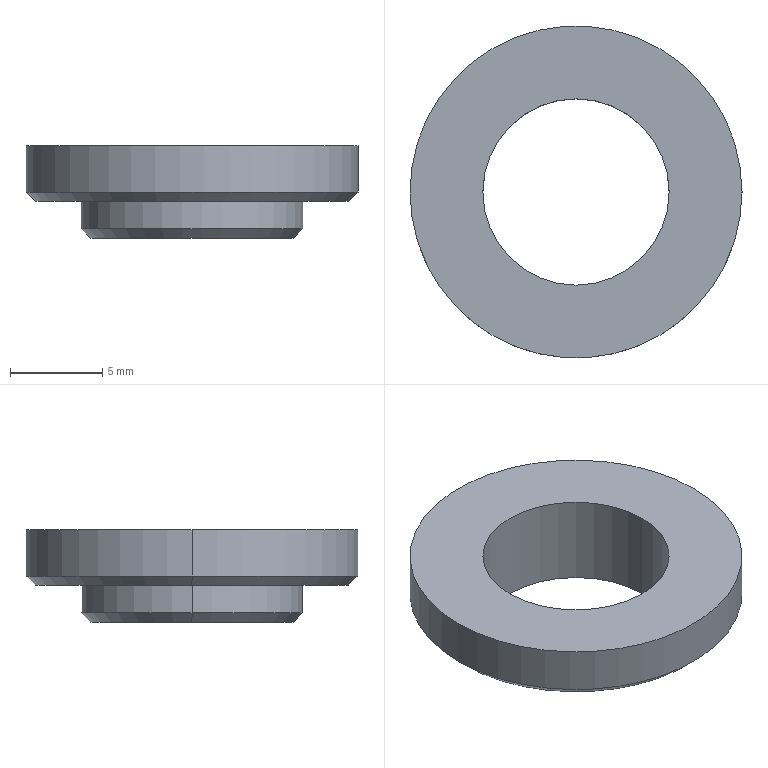Part | SolidWorks | features BaseBody 1 | 1 solid | 13 faces | box 18 x 18 x 5 mm | volume 577.49 mm3 | cylinder 6 | cone 4 | plane 3 | commonest cylinder face diameters 10.1 x2 12 x2 18 x2
STEP:
#1=CARTESIAN_POINT('',(-8.5,0.,2.));
#2=VERTEX_POINT('',#1);
#3=CARTESIAN_POINT('',(8.5,0.,2.));
#4=VERTEX_POINT('',#3);
#5=CARTESIAN_POINT('',(0.,0.,2.));
#6=DIRECTION('',(0.,0.,-1.));
#7=DIRECTION('',(-1.,0.,0.));
#8=AXIS2_PLACEMENT_3D('',#5,#6,#7);
#9=CIRCLE('',#8,8.5);
#10=EDGE_CURVE('',#2,#4,#9,.T.);
#11=ORIENTED_EDGE('',*,*,#10,.F.);
#12=CARTESIAN_POINT('',(-9.,0.,2.5));
#13=VERTEX_POINT('',#12);
#14=CARTESIAN_POINT('',(-8.5,0.,2.));
#15=DIRECTION('',(-0.7071,0.,0.7071));
#16=VECTOR('',#15,1000.);
#17=LINE('',#14,#16);
#18=EDGE_CURVE('',#2,#13,#17,.T.);
#19=ORIENTED_EDGE('',*,*,#18,.T.);
#20=CARTESIAN_POINT('',(9.,0.,2.5));
#21=VERTEX_POINT('',#20);
#22=CARTESIAN_POINT('',(0.,0.,2.5));
#23=DIRECTION('',(0.,0.,1.));
#24=DIRECTION('',(-1.,0.,0.));
#25=AXIS2_PLACEMENT_3D('',#22,#23,#24);
#26=CIRCLE('',#25,9.);
#27=EDGE_CURVE('',#21,#13,#26,.T.);
#28=ORIENTED_EDGE('',*,*,#27,.F.);
#29=CARTESIAN_POINT('',(8.5,0.,2.));
#30=DIRECTION('',(0.7071,0.,0.7071));
#31=VECTOR('',#30,1000.);
#32=LINE('',#29,#31);
#33=EDGE_CURVE('',#4,#21,#32,.T.);
#34=ORIENTED_EDGE('',*,*,#33,.F.);
#35=EDGE_LOOP('',(#11,#19,#28,#34));
#36=FACE_OUTER_BOUND('',#35,.T.);
#37=CARTESIAN_POINT('',(0.,0.,2.));
#38=DIRECTION('',(0.,0.,1.));
#39=DIRECTION('',(1.,0.,0.));
#40=AXIS2_PLACEMENT_3D('',#37,#38,#39);
#41=CONICAL_SURFACE('',#40,8.5,0.7854);
#42=ADVANCED_FACE('',(#36),#41,.T.);
#43=CARTESIAN_POINT('',(-5.5,0.,0.));
#44=VERTEX_POINT('',#43);
#45=CARTESIAN_POINT('',(5.5,0.,0.));
#46=VERTEX_POINT('',#45);
#47=CARTESIAN_POINT('',(0.,0.,0.));
#48=DIRECTION('',(0.,0.,-1.));
#49=DIRECTION('',(1.,0.,0.));
#50=AXIS2_PLACEMENT_3D('',#47,#48,#49);
#51=CIRCLE('',#50,5.5);
#52=EDGE_CURVE('',#44,#46,#51,.T.);
#53=ORIENTED_EDGE('',*,*,#52,.F.);
#54=CARTESIAN_POINT('',(-6.,0.,0.5));
#55=VERTEX_POINT('',#54);
#56=CARTESIAN_POINT('',(-5.5,0.,0.));
#57=DIRECTION('',(-0.7071,0.,0.7071));
#58=VECTOR('',#57,1000.);
#59=LINE('',#56,#58);
#60=EDGE_CURVE('',#44,#55,#59,.T.);
#61=ORIENTED_EDGE('',*,*,#60,.T.);
#62=CARTESIAN_POINT('',(6.,0.,0.5));
#63=VERTEX_POINT('',#62);
#64=CARTESIAN_POINT('',(0.,0.,0.5));
#65=DIRECTION('',(0.,0.,1.));
#66=DIRECTION('',(1.,0.,0.));
#67=AXIS2_PLACEMENT_3D('',#64,#65,#66);
#68=CIRCLE('',#67,6.);
#69=EDGE_CURVE('',#63,#55,#68,.T.);
#70=ORIENTED_EDGE('',*,*,#69,.F.);
#71=CARTESIAN_POINT('',(5.5,0.,0.));
#72=DIRECTION('',(0.7071,0.,0.7071));
#73=VECTOR('',#72,1000.);
#74=LINE('',#71,#73);
#75=EDGE_CURVE('',#46,#63,#74,.T.);
#76=ORIENTED_EDGE('',*,*,#75,.F.);
#77=EDGE_LOOP('',(#53,#61,#70,#76));
#78=FACE_OUTER_BOUND('',#77,.T.);
#79=CARTESIAN_POINT('',(0.,0.,0.));
#80=DIRECTION('',(0.,0.,1.));
#81=DIRECTION('',(1.,0.,0.));
#82=AXIS2_PLACEMENT_3D('',#79,#80,#81);
#83=CONICAL_SURFACE('',#82,5.5,0.7854);
#84=ADVANCED_FACE('',(#78),#83,.T.);
#85=CARTESIAN_POINT('',(-6.,0.,2.));
#86=VERTEX_POINT('',#85);
#87=CARTESIAN_POINT('',(6.,0.,2.));
#88=VERTEX_POINT('',#87);
#89=CARTESIAN_POINT('',(0.,0.,2.));
#90=DIRECTION('',(0.,0.,-1.));
#91=DIRECTION('',(-1.,0.,0.));
#92=AXIS2_PLACEMENT_3D('',#89,#90,#91);
#93=CIRCLE('',#92,6.);
#94=EDGE_CURVE('',#86,#88,#93,.T.);
#95=ORIENTED_EDGE('',*,*,#94,.T.);
#96=CARTESIAN_POINT('',(6.,0.,2.));
#97=DIRECTION('',(0.,0.,-1.));
#98=VECTOR('',#97,1000.);
#99=LINE('',#96,#98);
#100=EDGE_CURVE('',#88,#63,#99,.T.);
#101=ORIENTED_EDGE('',*,*,#100,.T.);
#102=ORIENTED_EDGE('',*,*,#69,.T.);
#103=CARTESIAN_POINT('',(-6.,0.,2.));
#104=DIRECTION('',(0.,0.,-1.));
#105=VECTOR('',#104,1000.);
#106=LINE('',#103,#105);
#107=EDGE_CURVE('',#86,#55,#106,.T.);
#108=ORIENTED_EDGE('',*,*,#107,.F.);
#109=EDGE_LOOP('',(#95,#101,#102,#108));
#110=FACE_OUTER_BOUND('',#109,.T.);
#111=CARTESIAN_POINT('',(0.,0.,2.));
#112=DIRECTION('',(0.,0.,-1.));
#113=DIRECTION('',(-1.,0.,0.));
#114=AXIS2_PLACEMENT_3D('',#111,#112,#113);
#115=CYLINDRICAL_SURFACE('',#114,6.);
#116=ADVANCED_FACE('',(#110),#115,.T.);
#117=CARTESIAN_POINT('',(-5.05,0.,5.));
#118=VERTEX_POINT('',#117);
#119=CARTESIAN_POINT('',(5.05,0.,5.));
#120=VERTEX_POINT('',#119);
#121=CARTESIAN_POINT('',(0.,0.,5.));
#122=DIRECTION('',(0.,0.,1.));
#123=DIRECTION('',(1.,0.,0.));
#124=AXIS2_PLACEMENT_3D('',#121,#122,#123);
#125=CIRCLE('',#124,5.05);
#126=EDGE_CURVE('',#118,#120,#125,.T.);
#127=ORIENTED_EDGE('',*,*,#126,.T.);
#128=CARTESIAN_POINT('',(5.05,0.,0.));
#129=VERTEX_POINT('',#128);
#130=CARTESIAN_POINT('',(5.05,0.,5.));
#131=DIRECTION('',(0.,0.,-1.));
#132=VECTOR('',#131,1000.);
#133=LINE('',#130,#132);
#134=EDGE_CURVE('',#120,#129,#133,.T.);
#135=ORIENTED_EDGE('',*,*,#134,.T.);
#136=CARTESIAN_POINT('',(-5.05,0.,0.));
#137=VERTEX_POINT('',#136);
#138=CARTESIAN_POINT('',(0.,0.,0.));
#139=DIRECTION('',(0.,0.,1.));
#140=DIRECTION('',(1.,0.,0.));
#141=AXIS2_PLACEMENT_3D('',#138,#139,#140);
#142=CIRCLE('',#141,5.05);
#143=EDGE_CURVE('',#137,#129,#142,.T.);
#144=ORIENTED_EDGE('',*,*,#143,.F.);
#145=CARTESIAN_POINT('',(-5.05,0.,5.));
#146=DIRECTION('',(0.,0.,-1.));
#147=VECTOR('',#146,1000.);
#148=LINE('',#145,#147);
#149=EDGE_CURVE('',#118,#137,#148,.T.);
#150=ORIENTED_EDGE('',*,*,#149,.F.);
#151=EDGE_LOOP('',(#127,#135,#144,#150));
#152=FACE_OUTER_BOUND('',#151,.T.);
#153=CARTESIAN_POINT('',(0.,0.,5.));
#154=DIRECTION('',(0.,0.,-1.));
#155=DIRECTION('',(-1.,0.,0.));
#156=AXIS2_PLACEMENT_3D('',#153,#154,#155);
#157=CYLINDRICAL_SURFACE('',#156,5.05);
#158=ADVANCED_FACE('',(#152),#157,.F.);
#159=CARTESIAN_POINT('',(9.,0.,5.));
#160=VERTEX_POINT('',#159);
#161=CARTESIAN_POINT('',(-9.,0.,5.));
#162=VERTEX_POINT('',#161);
#163=CARTESIAN_POINT('',(0.,0.,5.));
#164=DIRECTION('',(0.,0.,1.));
#165=DIRECTION('',(1.,0.,0.));
#166=AXIS2_PLACEMENT_3D('',#163,#164,#165);
#167=CIRCLE('',#166,9.);
#168=EDGE_CURVE('',#160,#162,#167,.T.);
#169=ORIENTED_EDGE('',*,*,#168,.F.);
#170=CARTESIAN_POINT('',(9.,0.,5.));
#171=DIRECTION('',(0.,0.,-1.));
#172=VECTOR('',#171,1000.);
#173=LINE('',#170,#172);
#174=EDGE_CURVE('',#160,#21,#173,.T.);
#175=ORIENTED_EDGE('',*,*,#174,.T.);
#176=ORIENTED_EDGE('',*,*,#27,.T.);
#177=CARTESIAN_POINT('',(-9.,0.,5.));
#178=DIRECTION('',(0.,0.,-1.));
#179=VECTOR('',#178,1000.);
#180=LINE('',#177,#179);
#181=EDGE_CURVE('',#162,#13,#180,.T.);
#182=ORIENTED_EDGE('',*,*,#181,.F.);
#183=EDGE_LOOP('',(#169,#175,#176,#182));
#184=FACE_OUTER_BOUND('',#183,.T.);
#185=CARTESIAN_POINT('',(0.,0.,5.));
#186=DIRECTION('',(0.,0.,-1.));
#187=DIRECTION('',(-1.,0.,0.));
#188=AXIS2_PLACEMENT_3D('',#185,#186,#187);
#189=CYLINDRICAL_SURFACE('',#188,9.);
#190=ADVANCED_FACE('',(#184),#189,.T.);
#191=ORIENTED_EDGE('',*,*,#94,.F.);
#192=CARTESIAN_POINT('',(0.,0.,2.));
#193=DIRECTION('',(0.,0.,-1.));
#194=DIRECTION('',(-1.,0.,0.));
#195=AXIS2_PLACEMENT_3D('',#192,#193,#194);
#196=CIRCLE('',#195,6.);
#197=EDGE_CURVE('',#88,#86,#196,.T.);
#198=ORIENTED_EDGE('',*,*,#197,.F.);
#199=EDGE_LOOP('',(#191,#198));
#200=FACE_BOUND('',#199,.T.);
#201=CARTESIAN_POINT('',(0.,0.,2.));
#202=DIRECTION('',(0.,0.,-1.));
#203=DIRECTION('',(-1.,0.,0.));
#204=AXIS2_PLACEMENT_3D('',#201,#202,#203);
#205=CIRCLE('',#204,8.5);
#206=EDGE_CURVE('',#4,#2,#205,.T.);
#207=ORIENTED_EDGE('',*,*,#206,.T.);
#208=ORIENTED_EDGE('',*,*,#10,.T.);
#209=EDGE_LOOP('',(#207,#208));
#210=FACE_OUTER_BOUND('',#209,.T.);
#211=CARTESIAN_POINT('',(0.,0.,2.));
#212=DIRECTION('',(0.,0.,-1.));
#213=DIRECTION('',(0.,-1.,0.));
#214=AXIS2_PLACEMENT_3D('',#211,#212,#213);
#215=PLANE('',#214);
#216=ADVANCED_FACE('',(#200,#210),#215,.T.);
#217=ORIENTED_EDGE('',*,*,#126,.F.);
#218=CARTESIAN_POINT('',(0.,0.,5.));
#219=DIRECTION('',(0.,0.,1.));
#220=DIRECTION('',(1.,0.,0.));
#221=AXIS2_PLACEMENT_3D('',#218,#219,#220);
#222=CIRCLE('',#221,5.05);
#223=EDGE_CURVE('',#120,#118,#222,.T.);
#224=ORIENTED_EDGE('',*,*,#223,.F.);
#225=EDGE_LOOP('',(#217,#224));
#226=FACE_BOUND('',#225,.T.);
#227=CARTESIAN_POINT('',(0.,0.,5.));
#228=DIRECTION('',(0.,0.,1.));
#229=DIRECTION('',(1.,0.,0.));
#230=AXIS2_PLACEMENT_3D('',#227,#228,#229);
#231=CIRCLE('',#230,9.);
#232=EDGE_CURVE('',#162,#160,#231,.T.);
#233=ORIENTED_EDGE('',*,*,#232,.T.);
#234=ORIENTED_EDGE('',*,*,#168,.T.);
#235=EDGE_LOOP('',(#233,#234));
#236=FACE_OUTER_BOUND('',#235,.T.);
#237=CARTESIAN_POINT('',(0.,0.,5.));
#238=DIRECTION('',(0.,0.,1.));
#239=DIRECTION('',(1.,0.,0.));
#240=AXIS2_PLACEMENT_3D('',#237,#238,#239);
#241=PLANE('',#240);
#242=ADVANCED_FACE('',(#226,#236),#241,.T.);
#243=ORIENTED_EDGE('',*,*,#143,.T.);
#244=CARTESIAN_POINT('',(0.,0.,0.));
#245=DIRECTION('',(0.,0.,1.));
#246=DIRECTION('',(1.,0.,0.));
#247=AXIS2_PLACEMENT_3D('',#244,#245,#246);
#248=CIRCLE('',#247,5.05);
#249=EDGE_CURVE('',#129,#137,#248,.T.);
#250=ORIENTED_EDGE('',*,*,#249,.T.);
#251=EDGE_LOOP('',(#243,#250));
#252=FACE_BOUND('',#251,.T.);
#253=CARTESIAN_POINT('',(0.,0.,0.));
#254=DIRECTION('',(0.,0.,-1.));
#255=DIRECTION('',(1.,0.,0.));
#256=AXIS2_PLACEMENT_3D('',#253,#254,#255);
#257=CIRCLE('',#256,5.5);
#258=EDGE_CURVE('',#46,#44,#257,.T.);
#259=ORIENTED_EDGE('',*,*,#258,.T.);
#260=ORIENTED_EDGE('',*,*,#52,.T.);
#261=EDGE_LOOP('',(#259,#260));
#262=FACE_OUTER_BOUND('',#261,.T.);
#263=CARTESIAN_POINT('',(0.,0.,0.));
#264=DIRECTION('',(0.,0.,1.));
#265=DIRECTION('',(1.,0.,0.));
#266=AXIS2_PLACEMENT_3D('',#263,#264,#265);
#267=PLANE('',#266);
#268=ADVANCED_FACE('',(#252,#262),#267,.F.);
#269=ORIENTED_EDGE('',*,*,#174,.F.);
#270=ORIENTED_EDGE('',*,*,#232,.F.);
#271=ORIENTED_EDGE('',*,*,#181,.T.);
#272=CARTESIAN_POINT('',(0.,0.,2.5));
#273=DIRECTION('',(0.,0.,1.));
#274=DIRECTION('',(-1.,0.,0.));
#275=AXIS2_PLACEMENT_3D('',#272,#273,#274);
#276=CIRCLE('',#275,9.);
#277=EDGE_CURVE('',#13,#21,#276,.T.);
#278=ORIENTED_EDGE('',*,*,#277,.T.);
#279=EDGE_LOOP('',(#269,#270,#271,#278));
#280=FACE_OUTER_BOUND('',#279,.T.);
#281=CARTESIAN_POINT('',(0.,0.,5.));
#282=DIRECTION('',(0.,0.,-1.));
#283=DIRECTION('',(-1.,0.,0.));
#284=AXIS2_PLACEMENT_3D('',#281,#282,#283);
#285=CYLINDRICAL_SURFACE('',#284,9.);
#286=ADVANCED_FACE('',(#280),#285,.T.);
#287=ORIENTED_EDGE('',*,*,#134,.F.);
#288=ORIENTED_EDGE('',*,*,#223,.T.);
#289=ORIENTED_EDGE('',*,*,#149,.T.);
#290=ORIENTED_EDGE('',*,*,#249,.F.);
#291=EDGE_LOOP('',(#287,#288,#289,#290));
#292=FACE_OUTER_BOUND('',#291,.T.);
#293=CARTESIAN_POINT('',(0.,0.,5.));
#294=DIRECTION('',(0.,0.,-1.));
#295=DIRECTION('',(-1.,0.,0.));
#296=AXIS2_PLACEMENT_3D('',#293,#294,#295);
#297=CYLINDRICAL_SURFACE('',#296,5.05);
#298=ADVANCED_FACE('',(#292),#297,.F.);
#299=ORIENTED_EDGE('',*,*,#100,.F.);
#300=ORIENTED_EDGE('',*,*,#197,.T.);
#301=ORIENTED_EDGE('',*,*,#107,.T.);
#302=CARTESIAN_POINT('',(0.,0.,0.5));
#303=DIRECTION('',(0.,0.,1.));
#304=DIRECTION('',(1.,0.,0.));
#305=AXIS2_PLACEMENT_3D('',#302,#303,#304);
#306=CIRCLE('',#305,6.);
#307=EDGE_CURVE('',#55,#63,#306,.T.);
#308=ORIENTED_EDGE('',*,*,#307,.T.);
#309=EDGE_LOOP('',(#299,#300,#301,#308));
#310=FACE_OUTER_BOUND('',#309,.T.);
#311=CARTESIAN_POINT('',(0.,0.,2.));
#312=DIRECTION('',(0.,0.,-1.));
#313=DIRECTION('',(-1.,0.,0.));
#314=AXIS2_PLACEMENT_3D('',#311,#312,#313);
#315=CYLINDRICAL_SURFACE('',#314,6.);
#316=ADVANCED_FACE('',(#310),#315,.T.);
#317=ORIENTED_EDGE('',*,*,#60,.F.);
#318=ORIENTED_EDGE('',*,*,#258,.F.);
#319=ORIENTED_EDGE('',*,*,#75,.T.);
#320=ORIENTED_EDGE('',*,*,#307,.F.);
#321=EDGE_LOOP('',(#317,#318,#319,#320));
#322=FACE_OUTER_BOUND('',#321,.T.);
#323=CARTESIAN_POINT('',(0.,0.,0.));
#324=DIRECTION('',(0.,0.,1.));
#325=DIRECTION('',(1.,0.,0.));
#326=AXIS2_PLACEMENT_3D('',#323,#324,#325);
#327=CONICAL_SURFACE('',#326,5.5,0.7854);
#328=ADVANCED_FACE('',(#322),#327,.T.);
#329=ORIENTED_EDGE('',*,*,#18,.F.);
#330=ORIENTED_EDGE('',*,*,#206,.F.);
#331=ORIENTED_EDGE('',*,*,#33,.T.);
#332=ORIENTED_EDGE('',*,*,#277,.F.);
#333=EDGE_LOOP('',(#329,#330,#331,#332));
#334=FACE_OUTER_BOUND('',#333,.T.);
#335=CARTESIAN_POINT('',(0.,0.,2.));
#336=DIRECTION('',(0.,0.,1.));
#337=DIRECTION('',(1.,0.,0.));
#338=AXIS2_PLACEMENT_3D('',#335,#336,#337);
#339=CONICAL_SURFACE('',#338,8.5,0.7854);
#340=ADVANCED_FACE('',(#334),#339,.T.);
#341=CLOSED_SHELL('',(#42,#84,#116,#158,#190,#216,#242,#268,#286,#298,#316,#328,#340));
#342=MANIFOLD_SOLID_BREP('',#341);
#343=CARTESIAN_POINT('',(0.,0.,0.));
#344=DIRECTION('',(0.,0.,1.));
#345=DIRECTION('',(1.,0.,0.));
#346=AXIS2_PLACEMENT_3D('',#343,#344,#345);
#347=(LENGTH_UNIT()NAMED_UNIT(*)SI_UNIT(.MILLI.,.METRE.));
#348=UNCERTAINTY_MEASURE_WITH_UNIT(LENGTH_MEASURE(0.00001),#347,'','');
#349=(NAMED_UNIT(*)PLANE_ANGLE_UNIT()SI_UNIT($,.RADIAN.));
#350=(NAMED_UNIT(*)SI_UNIT($,.STERADIAN.)SOLID_ANGLE_UNIT());
#351=(GEOMETRIC_REPRESENTATION_CONTEXT(3)GLOBAL_UNCERTAINTY_ASSIGNED_CONTEXT((#348))GLOBAL_UNIT_ASSIGNED_CONTEXT((#347,#349,#350))REPRESENTATION_CONTEXT('',''));
#352=ADVANCED_BREP_SHAPE_REPRESENTATION('',(#342,#346),#351);